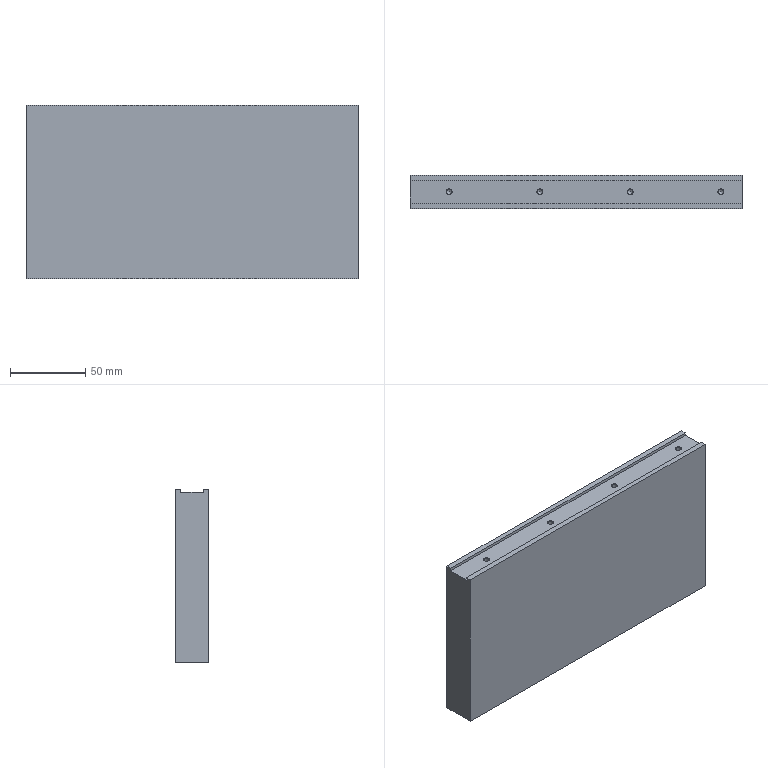Part | STEP file | Tube feed_id590_x_t | 1 solid | 22 faces | box 220 x 22 x 114.85 mm | volume 548747 mm3 | plane 10 | cone 8 | cylinder 4 | commonest cylinder face diameters 3.3 x4
STEP:
#1=CARTESIAN_POINT('',(0.,0.,0.));
#2=DIRECTION('',(0.,0.,1.));
#3=DIRECTION('',(1.,0.,0.));
#4=AXIS2_PLACEMENT_3D('',#1,#2,#3);
#5=CARTESIAN_POINT('',(21.,218.436,-89.15));
#6=VERTEX_POINT('',#5);
#7=CARTESIAN_POINT('',(21.,218.436,-91.15));
#8=VERTEX_POINT('',#7);
#9=CARTESIAN_POINT('',(21.,218.436,-89.969));
#10=DIRECTION('',(0.,0.,-1.));
#11=VECTOR('',#10,1.);
#12=LINE('',#9,#11);
#13=CARTESIAN_POINT('',(21.,221.936,-134.));
#14=DIRECTION('',(1.,0.,0.));
#15=DIRECTION('',(0.,0.,-1.));
#16=AXIS2_PLACEMENT_3D('',#13,#14,#15);
#17=PLANE('',#16);
#18=CARTESIAN_POINT('',(-44.031,-3.5));
#19=DIRECTION('',(1.,0.));
#20=VECTOR('',#19,1.);
#21=LINE('',#18,#20);
#22=(GEOMETRIC_REPRESENTATION_CONTEXT(2)PARAMETRIC_REPRESENTATION_CONTEXT()REPRESENTATION_CONTEXT('',''));
#23=DEFINITIONAL_REPRESENTATION('',(#21),#22);
#24=PCURVE('',#17,#23);
#25=CARTESIAN_POINT('',(1092.73,218.436,-89.969));
#26=DIRECTION('',(0.,1.,0.));
#27=DIRECTION('',(0.,0.,1.));
#28=AXIS2_PLACEMENT_3D('',#25,#26,#27);
#29=PLANE('',#28);
#30=CARTESIAN_POINT('',(0.,-1071.73));
#31=DIRECTION('',(-1.,0.));
#32=VECTOR('',#31,1.);
#33=LINE('',#30,#32);
#34=(GEOMETRIC_REPRESENTATION_CONTEXT(2)PARAMETRIC_REPRESENTATION_CONTEXT()REPRESENTATION_CONTEXT('',''));
#35=DEFINITIONAL_REPRESENTATION('',(#33),#34);
#36=PCURVE('',#29,#35);
#37=SURFACE_CURVE('',#12,(#24,#36),.PCURVE_S1.);
#38=EDGE_CURVE('',#6,#8,#37,.T.);
#39=ORIENTED_EDGE('',*,*,#38,.F.);
#40=CARTESIAN_POINT('',(21.,221.936,-89.15));
#41=VERTEX_POINT('',#40);
#42=CARTESIAN_POINT('',(21.,221.936,-89.15));
#43=DIRECTION('',(0.,-1.,0.));
#44=VECTOR('',#43,1.);
#45=LINE('',#42,#44);
#46=CARTESIAN_POINT('',(-44.85,0.));
#47=DIRECTION('',(0.,-1.));
#48=VECTOR('',#47,1.);
#49=LINE('',#46,#48);
#50=(GEOMETRIC_REPRESENTATION_CONTEXT(2)PARAMETRIC_REPRESENTATION_CONTEXT()REPRESENTATION_CONTEXT('',''));
#51=DEFINITIONAL_REPRESENTATION('',(#49),#50);
#52=PCURVE('',#17,#51);
#53=CARTESIAN_POINT('',(1092.73,218.436,-89.15));
#54=DIRECTION('',(0.,0.,-1.));
#55=DIRECTION('',(-1.,0.,0.));
#56=AXIS2_PLACEMENT_3D('',#53,#54,#55);
#57=PLANE('',#56);
#58=CARTESIAN_POINT('',(1071.73,3.5));
#59=DIRECTION('',(0.,-1.));
#60=VECTOR('',#59,1.);
#61=LINE('',#58,#60);
#62=(GEOMETRIC_REPRESENTATION_CONTEXT(2)PARAMETRIC_REPRESENTATION_CONTEXT()REPRESENTATION_CONTEXT('',''));
#63=DEFINITIONAL_REPRESENTATION('',(#61),#62);
#64=PCURVE('',#57,#63);
#65=SURFACE_CURVE('',#45,(#52,#64),.PCURVE_S1.);
#66=EDGE_CURVE('',#41,#6,#65,.T.);
#67=ORIENTED_EDGE('',*,*,#66,.F.);
#68=CARTESIAN_POINT('',(21.,221.936,-204.));
#69=VERTEX_POINT('',#68);
#70=CARTESIAN_POINT('',(21.,221.936,-134.));
#71=DIRECTION('',(0.,0.,-1.));
#72=VECTOR('',#71,1.);
#73=LINE('',#70,#72);
#74=CARTESIAN_POINT('',(0.,0.));
#75=DIRECTION('',(1.,0.));
#76=VECTOR('',#75,1.);
#77=LINE('',#74,#76);
#78=(GEOMETRIC_REPRESENTATION_CONTEXT(2)PARAMETRIC_REPRESENTATION_CONTEXT()REPRESENTATION_CONTEXT('',''));
#79=DEFINITIONAL_REPRESENTATION('',(#77),#78);
#80=PCURVE('',#17,#79);
#81=CARTESIAN_POINT('',(241.,221.936,-134.));
#82=DIRECTION('',(0.,-1.,0.));
#83=DIRECTION('',(0.,0.,-1.));
#84=AXIS2_PLACEMENT_3D('',#81,#82,#83);
#85=PLANE('',#84);
#86=CARTESIAN_POINT('',(0.,-220.));
#87=DIRECTION('',(1.,0.));
#88=VECTOR('',#87,1.);
#89=LINE('',#86,#88);
#90=(GEOMETRIC_REPRESENTATION_CONTEXT(2)PARAMETRIC_REPRESENTATION_CONTEXT()REPRESENTATION_CONTEXT('',''));
#91=DEFINITIONAL_REPRESENTATION('',(#89),#90);
#92=PCURVE('',#85,#91);
#93=SURFACE_CURVE('',#73,(#80,#92),.PCURVE_S1.);
#94=EDGE_CURVE('',#41,#69,#93,.T.);
#95=ORIENTED_EDGE('',*,*,#94,.T.);
#96=CARTESIAN_POINT('',(21.,199.936,-204.));
#97=VERTEX_POINT('',#96);
#98=CARTESIAN_POINT('',(21.,221.936,-204.));
#99=DIRECTION('',(0.,-1.,0.));
#100=VECTOR('',#99,1.);
#101=LINE('',#98,#100);
#102=CARTESIAN_POINT('',(70.,0.));
#103=DIRECTION('',(0.,-1.));
#104=VECTOR('',#103,1.);
#105=LINE('',#102,#104);
#106=(GEOMETRIC_REPRESENTATION_CONTEXT(2)PARAMETRIC_REPRESENTATION_CONTEXT()REPRESENTATION_CONTEXT('',''));
#107=DEFINITIONAL_REPRESENTATION('',(#105),#106);
#108=PCURVE('',#17,#107);
#109=CARTESIAN_POINT('',(0.,0.,-204.));
#110=DIRECTION('',(0.,0.,1.));
#111=DIRECTION('',(1.,0.,0.));
#112=AXIS2_PLACEMENT_3D('',#109,#110,#111);
#113=PLANE('',#112);
#114=CARTESIAN_POINT('',(21.,221.936));
#115=DIRECTION('',(0.,-1.));
#116=VECTOR('',#115,1.);
#117=LINE('',#114,#116);
#118=(GEOMETRIC_REPRESENTATION_CONTEXT(2)PARAMETRIC_REPRESENTATION_CONTEXT()REPRESENTATION_CONTEXT('',''));
#119=DEFINITIONAL_REPRESENTATION('',(#117),#118);
#120=PCURVE('',#113,#119);
#121=SURFACE_CURVE('',#101,(#108,#120),.PCURVE_S1.);
#122=EDGE_CURVE('',#69,#97,#121,.T.);
#123=ORIENTED_EDGE('',*,*,#122,.T.);
#124=CARTESIAN_POINT('',(21.,199.936,-89.15));
#125=VERTEX_POINT('',#124);
#126=CARTESIAN_POINT('',(21.,199.936,-134.));
#127=DIRECTION('',(0.,0.,-1.));
#128=VECTOR('',#127,1.);
#129=LINE('',#126,#128);
#130=CARTESIAN_POINT('',(0.,-22.));
#131=DIRECTION('',(1.,0.));
#132=VECTOR('',#131,1.);
#133=LINE('',#130,#132);
#134=(GEOMETRIC_REPRESENTATION_CONTEXT(2)PARAMETRIC_REPRESENTATION_CONTEXT()REPRESENTATION_CONTEXT('',''));
#135=DEFINITIONAL_REPRESENTATION('',(#133),#134);
#136=PCURVE('',#17,#135);
#137=CARTESIAN_POINT('',(21.,199.936,-134.));
#138=DIRECTION('',(0.,1.,0.));
#139=DIRECTION('',(0.,0.,1.));
#140=AXIS2_PLACEMENT_3D('',#137,#138,#139);
#141=PLANE('',#140);
#142=CARTESIAN_POINT('',(0.,0.));
#143=DIRECTION('',(-1.,0.));
#144=VECTOR('',#143,1.);
#145=LINE('',#142,#144);
#146=(GEOMETRIC_REPRESENTATION_CONTEXT(2)PARAMETRIC_REPRESENTATION_CONTEXT()REPRESENTATION_CONTEXT('',''));
#147=DEFINITIONAL_REPRESENTATION('',(#145),#146);
#148=PCURVE('',#141,#147);
#149=SURFACE_CURVE('',#129,(#136,#148),.PCURVE_S1.);
#150=EDGE_CURVE('',#125,#97,#149,.T.);
#151=ORIENTED_EDGE('',*,*,#150,.F.);
#152=CARTESIAN_POINT('',(21.,203.436,-89.15));
#153=VERTEX_POINT('',#152);
#154=CARTESIAN_POINT('',(21.,221.936,-89.15));
#155=DIRECTION('',(0.,-1.,0.));
#156=VECTOR('',#155,1.);
#157=LINE('',#154,#156);
#158=CARTESIAN_POINT('',(-44.85,0.));
#159=DIRECTION('',(0.,-1.));
#160=VECTOR('',#159,1.);
#161=LINE('',#158,#160);
#162=(GEOMETRIC_REPRESENTATION_CONTEXT(2)PARAMETRIC_REPRESENTATION_CONTEXT()REPRESENTATION_CONTEXT('',''));
#163=DEFINITIONAL_REPRESENTATION('',(#161),#162);
#164=PCURVE('',#17,#163);
#165=CARTESIAN_POINT('',(1092.73,218.436,-89.15));
#166=DIRECTION('',(0.,0.,-1.));
#167=DIRECTION('',(-1.,0.,0.));
#168=AXIS2_PLACEMENT_3D('',#165,#166,#167);
#169=PLANE('',#168);
#170=CARTESIAN_POINT('',(1071.73,3.5));
#171=DIRECTION('',(0.,-1.));
#172=VECTOR('',#171,1.);
#173=LINE('',#170,#172);
#174=(GEOMETRIC_REPRESENTATION_CONTEXT(2)PARAMETRIC_REPRESENTATION_CONTEXT()REPRESENTATION_CONTEXT('',''));
#175=DEFINITIONAL_REPRESENTATION('',(#173),#174);
#176=PCURVE('',#169,#175);
#177=SURFACE_CURVE('',#157,(#164,#176),.PCURVE_S1.);
#178=EDGE_CURVE('',#153,#125,#177,.T.);
#179=ORIENTED_EDGE('',*,*,#178,.F.);
#180=CARTESIAN_POINT('',(21.,203.436,-91.15));
#181=VERTEX_POINT('',#180);
#182=CARTESIAN_POINT('',(21.,203.436,-91.15));
#183=DIRECTION('',(0.,0.,1.));
#184=VECTOR('',#183,1.);
#185=LINE('',#182,#184);
#186=CARTESIAN_POINT('',(-42.85,-18.5));
#187=DIRECTION('',(-1.,0.));
#188=VECTOR('',#187,1.);
#189=LINE('',#186,#188);
#190=(GEOMETRIC_REPRESENTATION_CONTEXT(2)PARAMETRIC_REPRESENTATION_CONTEXT()REPRESENTATION_CONTEXT('',''));
#191=DEFINITIONAL_REPRESENTATION('',(#189),#190);
#192=PCURVE('',#17,#191);
#193=CARTESIAN_POINT('',(1092.73,203.436,-91.15));
#194=DIRECTION('',(0.,-1.,0.));
#195=DIRECTION('',(0.,0.,-1.));
#196=AXIS2_PLACEMENT_3D('',#193,#194,#195);
#197=PLANE('',#196);
#198=CARTESIAN_POINT('',(0.,-1071.73));
#199=DIRECTION('',(-1.,0.));
#200=VECTOR('',#199,1.);
#201=LINE('',#198,#200);
#202=(GEOMETRIC_REPRESENTATION_CONTEXT(2)PARAMETRIC_REPRESENTATION_CONTEXT()REPRESENTATION_CONTEXT('',''));
#203=DEFINITIONAL_REPRESENTATION('',(#201),#202);
#204=PCURVE('',#197,#203);
#205=SURFACE_CURVE('',#185,(#192,#204),.PCURVE_S1.);
#206=EDGE_CURVE('',#181,#153,#205,.T.);
#207=ORIENTED_EDGE('',*,*,#206,.F.);
#208=CARTESIAN_POINT('',(21.,218.436,-91.15));
#209=DIRECTION('',(0.,-1.,0.));
#210=VECTOR('',#209,1.);
#211=LINE('',#208,#210);
#212=CARTESIAN_POINT('',(-42.85,-3.5));
#213=DIRECTION('',(0.,-1.));
#214=VECTOR('',#213,1.);
#215=LINE('',#212,#214);
#216=(GEOMETRIC_REPRESENTATION_CONTEXT(2)PARAMETRIC_REPRESENTATION_CONTEXT()REPRESENTATION_CONTEXT('',''));
#217=DEFINITIONAL_REPRESENTATION('',(#215),#216);
#218=PCURVE('',#17,#217);
#219=CARTESIAN_POINT('',(1092.73,218.436,-91.15));
#220=DIRECTION('',(0.,0.,-1.));
#221=DIRECTION('',(-1.,0.,0.));
#222=AXIS2_PLACEMENT_3D('',#219,#220,#221);
#223=PLANE('',#222);
#224=CARTESIAN_POINT('',(1071.73,0.));
#225=DIRECTION('',(0.,-1.));
#226=VECTOR('',#225,1.);
#227=LINE('',#224,#226);
#228=(GEOMETRIC_REPRESENTATION_CONTEXT(2)PARAMETRIC_REPRESENTATION_CONTEXT()REPRESENTATION_CONTEXT('',''));
#229=DEFINITIONAL_REPRESENTATION('',(#227),#228);
#230=PCURVE('',#223,#229);
#231=SURFACE_CURVE('',#211,(#218,#230),.PCURVE_S1.);
#232=EDGE_CURVE('',#8,#181,#231,.T.);
#233=ORIENTED_EDGE('',*,*,#232,.F.);
#234=EDGE_LOOP('',(#39,#67,#95,#123,#151,#179,#207,#233));
#235=FACE_BOUND('',#234,.T.);
#236=ADVANCED_FACE('',(#235),#17,.F.);
#237=CARTESIAN_POINT('',(241.,203.436,-89.15));
#238=VERTEX_POINT('',#237);
#239=CARTESIAN_POINT('',(241.,203.436,-91.15));
#240=VERTEX_POINT('',#239);
#241=CARTESIAN_POINT('',(241.,203.436,-91.15));
#242=DIRECTION('',(0.,0.,-1.));
#243=VECTOR('',#242,1.);
#244=LINE('',#241,#243);
#245=CARTESIAN_POINT('',(241.,199.936,-134.));
#246=DIRECTION('',(-1.,0.,0.));
#247=DIRECTION('',(0.,0.,1.));
#248=AXIS2_PLACEMENT_3D('',#245,#246,#247);
#249=PLANE('',#248);
#250=CARTESIAN_POINT('',(42.85,3.5));
#251=DIRECTION('',(-1.,0.));
#252=VECTOR('',#251,1.);
#253=LINE('',#250,#252);
#254=(GEOMETRIC_REPRESENTATION_CONTEXT(2)PARAMETRIC_REPRESENTATION_CONTEXT()REPRESENTATION_CONTEXT('',''));
#255=DEFINITIONAL_REPRESENTATION('',(#253),#254);
#256=PCURVE('',#249,#255);
#257=CARTESIAN_POINT('',(0.,-851.73));
#258=DIRECTION('',(1.,0.));
#259=VECTOR('',#258,1.);
#260=LINE('',#257,#259);
#261=(GEOMETRIC_REPRESENTATION_CONTEXT(2)PARAMETRIC_REPRESENTATION_CONTEXT()REPRESENTATION_CONTEXT('',''));
#262=DEFINITIONAL_REPRESENTATION('',(#260),#261);
#263=PCURVE('',#197,#262);
#264=SURFACE_CURVE('',#244,(#256,#263),.PCURVE_S1.);
#265=EDGE_CURVE('',#238,#240,#264,.T.);
#266=ORIENTED_EDGE('',*,*,#265,.F.);
#267=CARTESIAN_POINT('',(241.,199.936,-89.15));
#268=VERTEX_POINT('',#267);
#269=CARTESIAN_POINT('',(241.,199.936,-89.15));
#270=DIRECTION('',(0.,1.,0.));
#271=VECTOR('',#270,1.);
#272=LINE('',#269,#271);
#273=CARTESIAN_POINT('',(44.85,0.));
#274=DIRECTION('',(0.,1.));
#275=VECTOR('',#274,1.);
#276=LINE('',#273,#275);
#277=(GEOMETRIC_REPRESENTATION_CONTEXT(2)PARAMETRIC_REPRESENTATION_CONTEXT()REPRESENTATION_CONTEXT('',''));
#278=DEFINITIONAL_REPRESENTATION('',(#276),#277);
#279=PCURVE('',#249,#278);
#280=CARTESIAN_POINT('',(851.73,-18.5));
#281=DIRECTION('',(0.,1.));
#282=VECTOR('',#281,1.);
#283=LINE('',#280,#282);
#284=(GEOMETRIC_REPRESENTATION_CONTEXT(2)PARAMETRIC_REPRESENTATION_CONTEXT()REPRESENTATION_CONTEXT('',''));
#285=DEFINITIONAL_REPRESENTATION('',(#283),#284);
#286=PCURVE('',#169,#285);
#287=SURFACE_CURVE('',#272,(#279,#286),.PCURVE_S1.);
#288=EDGE_CURVE('',#268,#238,#287,.T.);
#289=ORIENTED_EDGE('',*,*,#288,.F.);
#290=CARTESIAN_POINT('',(241.,199.936,-204.));
#291=VERTEX_POINT('',#290);
#292=CARTESIAN_POINT('',(241.,199.936,-134.));
#293=DIRECTION('',(0.,0.,-1.));
#294=VECTOR('',#293,1.);
#295=LINE('',#292,#294);
#296=CARTESIAN_POINT('',(0.,0.));
#297=DIRECTION('',(-1.,0.));
#298=VECTOR('',#297,1.);
#299=LINE('',#296,#298);
#300=(GEOMETRIC_REPRESENTATION_CONTEXT(2)PARAMETRIC_REPRESENTATION_CONTEXT()REPRESENTATION_CONTEXT('',''));
#301=DEFINITIONAL_REPRESENTATION('',(#299),#300);
#302=PCURVE('',#249,#301);
#303=CARTESIAN_POINT('',(0.,220.));
#304=DIRECTION('',(-1.,0.));
#305=VECTOR('',#304,1.);
#306=LINE('',#303,#305);
#307=(GEOMETRIC_REPRESENTATION_CONTEXT(2)PARAMETRIC_REPRESENTATION_CONTEXT()REPRESENTATION_CONTEXT('',''));
#308=DEFINITIONAL_REPRESENTATION('',(#306),#307);
#309=PCURVE('',#141,#308);
#310=SURFACE_CURVE('',#295,(#302,#309),.PCURVE_S1.);
#311=EDGE_CURVE('',#268,#291,#310,.T.);
#312=ORIENTED_EDGE('',*,*,#311,.T.);
#313=CARTESIAN_POINT('',(241.,221.936,-204.));
#314=VERTEX_POINT('',#313);
#315=CARTESIAN_POINT('',(241.,199.936,-204.));
#316=DIRECTION('',(0.,1.,0.));
#317=VECTOR('',#316,1.);
#318=LINE('',#315,#317);
#319=CARTESIAN_POINT('',(-70.,0.));
#320=DIRECTION('',(0.,1.));
#321=VECTOR('',#320,1.);
#322=LINE('',#319,#321);
#323=(GEOMETRIC_REPRESENTATION_CONTEXT(2)PARAMETRIC_REPRESENTATION_CONTEXT()REPRESENTATION_CONTEXT('',''));
#324=DEFINITIONAL_REPRESENTATION('',(#322),#323);
#325=PCURVE('',#249,#324);
#326=CARTESIAN_POINT('',(241.,199.936));
#327=DIRECTION('',(0.,1.));
#328=VECTOR('',#327,1.);
#329=LINE('',#326,#328);
#330=(GEOMETRIC_REPRESENTATION_CONTEXT(2)PARAMETRIC_REPRESENTATION_CONTEXT()REPRESENTATION_CONTEXT('',''));
#331=DEFINITIONAL_REPRESENTATION('',(#329),#330);
#332=PCURVE('',#113,#331);
#333=SURFACE_CURVE('',#318,(#325,#332),.PCURVE_S1.);
#334=EDGE_CURVE('',#291,#314,#333,.T.);
#335=ORIENTED_EDGE('',*,*,#334,.T.);
#336=CARTESIAN_POINT('',(241.,221.936,-89.15));
#337=VERTEX_POINT('',#336);
#338=CARTESIAN_POINT('',(241.,221.936,-134.));
#339=DIRECTION('',(0.,0.,-1.));
#340=VECTOR('',#339,1.);
#341=LINE('',#338,#340);
#342=CARTESIAN_POINT('',(0.,22.));
#343=DIRECTION('',(-1.,0.));
#344=VECTOR('',#343,1.);
#345=LINE('',#342,#344);
#346=(GEOMETRIC_REPRESENTATION_CONTEXT(2)PARAMETRIC_REPRESENTATION_CONTEXT()REPRESENTATION_CONTEXT('',''));
#347=DEFINITIONAL_REPRESENTATION('',(#345),#346);
#348=PCURVE('',#249,#347);
#349=CARTESIAN_POINT('',(0.,0.));
#350=DIRECTION('',(1.,0.));
#351=VECTOR('',#350,1.);
#352=LINE('',#349,#351);
#353=(GEOMETRIC_REPRESENTATION_CONTEXT(2)PARAMETRIC_REPRESENTATION_CONTEXT()REPRESENTATION_CONTEXT('',''));
#354=DEFINITIONAL_REPRESENTATION('',(#352),#353);
#355=PCURVE('',#85,#354);
#356=SURFACE_CURVE('',#341,(#348,#355),.PCURVE_S1.);
#357=EDGE_CURVE('',#337,#314,#356,.T.);
#358=ORIENTED_EDGE('',*,*,#357,.F.);
#359=CARTESIAN_POINT('',(241.,218.436,-89.15));
#360=VERTEX_POINT('',#359);
#361=CARTESIAN_POINT('',(241.,199.936,-89.15));
#362=DIRECTION('',(0.,1.,0.));
#363=VECTOR('',#362,1.);
#364=LINE('',#361,#363);
#365=CARTESIAN_POINT('',(44.85,0.));
#366=DIRECTION('',(0.,1.));
#367=VECTOR('',#366,1.);
#368=LINE('',#365,#367);
#369=(GEOMETRIC_REPRESENTATION_CONTEXT(2)PARAMETRIC_REPRESENTATION_CONTEXT()REPRESENTATION_CONTEXT('',''));
#370=DEFINITIONAL_REPRESENTATION('',(#368),#369);
#371=PCURVE('',#249,#370);
#372=CARTESIAN_POINT('',(851.73,-18.5));
#373=DIRECTION('',(0.,1.));
#374=VECTOR('',#373,1.);
#375=LINE('',#372,#374);
#376=(GEOMETRIC_REPRESENTATION_CONTEXT(2)PARAMETRIC_REPRESENTATION_CONTEXT()REPRESENTATION_CONTEXT('',''));
#377=DEFINITIONAL_REPRESENTATION('',(#375),#376);
#378=PCURVE('',#57,#377);
#379=SURFACE_CURVE('',#364,(#371,#378),.PCURVE_S1.);
#380=EDGE_CURVE('',#360,#337,#379,.T.);
#381=ORIENTED_EDGE('',*,*,#380,.F.);
#382=CARTESIAN_POINT('',(241.,218.436,-91.15));
#383=VERTEX_POINT('',#382);
#384=CARTESIAN_POINT('',(241.,218.436,-89.969));
#385=DIRECTION('',(0.,0.,1.));
#386=VECTOR('',#385,1.);
#387=LINE('',#384,#386);
#388=CARTESIAN_POINT('',(44.031,18.5));
#389=DIRECTION('',(1.,0.));
#390=VECTOR('',#389,1.);
#391=LINE('',#388,#390);
#392=(GEOMETRIC_REPRESENTATION_CONTEXT(2)PARAMETRIC_REPRESENTATION_CONTEXT()REPRESENTATION_CONTEXT('',''));
#393=DEFINITIONAL_REPRESENTATION('',(#391),#392);
#394=PCURVE('',#249,#393);
#395=CARTESIAN_POINT('',(0.,-851.73));
#396=DIRECTION('',(1.,0.));
#397=VECTOR('',#396,1.);
#398=LINE('',#395,#397);
#399=(GEOMETRIC_REPRESENTATION_CONTEXT(2)PARAMETRIC_REPRESENTATION_CONTEXT()REPRESENTATION_CONTEXT('',''));
#400=DEFINITIONAL_REPRESENTATION('',(#398),#399);
#401=PCURVE('',#29,#400);
#402=SURFACE_CURVE('',#387,(#394,#401),.PCURVE_S1.);
#403=EDGE_CURVE('',#383,#360,#402,.T.);
#404=ORIENTED_EDGE('',*,*,#403,.F.);
#405=CARTESIAN_POINT('',(241.,218.436,-91.15));
#406=DIRECTION('',(0.,1.,0.));
#407=VECTOR('',#406,1.);
#408=LINE('',#405,#407);
#409=CARTESIAN_POINT('',(42.85,18.5));
#410=DIRECTION('',(0.,1.));
#411=VECTOR('',#410,1.);
#412=LINE('',#409,#411);
#413=(GEOMETRIC_REPRESENTATION_CONTEXT(2)PARAMETRIC_REPRESENTATION_CONTEXT()REPRESENTATION_CONTEXT('',''));
#414=DEFINITIONAL_REPRESENTATION('',(#412),#413);
#415=PCURVE('',#249,#414);
#416=CARTESIAN_POINT('',(851.73,0.));
#417=DIRECTION('',(0.,1.));
#418=VECTOR('',#417,1.);
#419=LINE('',#416,#418);
#420=(GEOMETRIC_REPRESENTATION_CONTEXT(2)PARAMETRIC_REPRESENTATION_CONTEXT()REPRESENTATION_CONTEXT('',''));
#421=DEFINITIONAL_REPRESENTATION('',(#419),#420);
#422=PCURVE('',#223,#421);
#423=SURFACE_CURVE('',#408,(#415,#422),.PCURVE_S1.);
#424=EDGE_CURVE('',#240,#383,#423,.T.);
#425=ORIENTED_EDGE('',*,*,#424,.F.);
#426=EDGE_LOOP('',(#266,#289,#312,#335,#358,#381,#404,#425));
#427=FACE_BOUND('',#426,.T.);
#428=ADVANCED_FACE('',(#427),#249,.F.);
#429=CARTESIAN_POINT('',(1092.73,203.436,-89.15));
#430=DIRECTION('',(1.,0.,0.));
#431=VECTOR('',#430,1.);
#432=LINE('',#429,#431);
#433=CARTESIAN_POINT('',(0.,-15.));
#434=DIRECTION('',(-1.,0.));
#435=VECTOR('',#434,1.);
#436=LINE('',#433,#435);
#437=(GEOMETRIC_REPRESENTATION_CONTEXT(2)PARAMETRIC_REPRESENTATION_CONTEXT()REPRESENTATION_CONTEXT('',''));
#438=DEFINITIONAL_REPRESENTATION('',(#436),#437);
#439=PCURVE('',#169,#438);
#440=CARTESIAN_POINT('',(-2.,0.));
#441=DIRECTION('',(0.,1.));
#442=VECTOR('',#441,1.);
#443=LINE('',#440,#442);
#444=(GEOMETRIC_REPRESENTATION_CONTEXT(2)PARAMETRIC_REPRESENTATION_CONTEXT()REPRESENTATION_CONTEXT('',''));
#445=DEFINITIONAL_REPRESENTATION('',(#443),#444);
#446=PCURVE('',#197,#445);
#447=SURFACE_CURVE('',#432,(#439,#446),.PCURVE_S1.);
#448=EDGE_CURVE('',#153,#238,#447,.T.);
#449=ORIENTED_EDGE('',*,*,#448,.F.);
#450=ORIENTED_EDGE('',*,*,#178,.T.);
#451=CARTESIAN_POINT('',(21.,199.936,-89.15));
#452=DIRECTION('',(1.,0.,0.));
#453=VECTOR('',#452,1.);
#454=LINE('',#451,#453);
#455=CARTESIAN_POINT('',(1071.73,-18.5));
#456=DIRECTION('',(-1.,0.));
#457=VECTOR('',#456,1.);
#458=LINE('',#455,#457);
#459=(GEOMETRIC_REPRESENTATION_CONTEXT(2)PARAMETRIC_REPRESENTATION_CONTEXT()REPRESENTATION_CONTEXT('',''));
#460=DEFINITIONAL_REPRESENTATION('',(#458),#459);
#461=PCURVE('',#169,#460);
#462=CARTESIAN_POINT('',(44.85,0.));
#463=DIRECTION('',(0.,1.));
#464=VECTOR('',#463,1.);
#465=LINE('',#462,#464);
#466=(GEOMETRIC_REPRESENTATION_CONTEXT(2)PARAMETRIC_REPRESENTATION_CONTEXT()REPRESENTATION_CONTEXT('',''));
#467=DEFINITIONAL_REPRESENTATION('',(#465),#466);
#468=PCURVE('',#141,#467);
#469=SURFACE_CURVE('',#454,(#461,#468),.PCURVE_S1.);
#470=EDGE_CURVE('',#125,#268,#469,.T.);
#471=ORIENTED_EDGE('',*,*,#470,.T.);
#472=ORIENTED_EDGE('',*,*,#288,.T.);
#473=EDGE_LOOP('',(#449,#450,#471,#472));
#474=FACE_BOUND('',#473,.T.);
#475=ADVANCED_FACE('',(#474),#169,.F.);
#476=CARTESIAN_POINT('',(21.,199.936,-204.));
#477=DIRECTION('',(1.,0.,0.));
#478=VECTOR('',#477,1.);
#479=LINE('',#476,#478);
#480=CARTESIAN_POINT('',(-70.,0.));
#481=DIRECTION('',(0.,1.));
#482=VECTOR('',#481,1.);
#483=LINE('',#480,#482);
#484=(GEOMETRIC_REPRESENTATION_CONTEXT(2)PARAMETRIC_REPRESENTATION_CONTEXT()REPRESENTATION_CONTEXT('',''));
#485=DEFINITIONAL_REPRESENTATION('',(#483),#484);
#486=PCURVE('',#141,#485);
#487=CARTESIAN_POINT('',(21.,199.936));
#488=DIRECTION('',(1.,0.));
#489=VECTOR('',#488,1.);
#490=LINE('',#487,#489);
#491=(GEOMETRIC_REPRESENTATION_CONTEXT(2)PARAMETRIC_REPRESENTATION_CONTEXT()REPRESENTATION_CONTEXT('',''));
#492=DEFINITIONAL_REPRESENTATION('',(#490),#491);
#493=PCURVE('',#113,#492);
#494=SURFACE_CURVE('',#479,(#486,#493),.PCURVE_S1.);
#495=EDGE_CURVE('',#97,#291,#494,.T.);
#496=ORIENTED_EDGE('',*,*,#495,.T.);
#497=ORIENTED_EDGE('',*,*,#311,.F.);
#498=ORIENTED_EDGE('',*,*,#470,.F.);
#499=ORIENTED_EDGE('',*,*,#150,.T.);
#500=EDGE_LOOP('',(#496,#497,#498,#499));
#501=FACE_BOUND('',#500,.T.);
#502=ADVANCED_FACE('',(#501),#141,.F.);
#503=CARTESIAN_POINT('',(241.,221.936,-204.));
#504=DIRECTION('',(-1.,0.,0.));
#505=VECTOR('',#504,1.);
#506=LINE('',#503,#505);
#507=CARTESIAN_POINT('',(70.,0.));
#508=DIRECTION('',(0.,-1.));
#509=VECTOR('',#508,1.);
#510=LINE('',#507,#509);
#511=(GEOMETRIC_REPRESENTATION_CONTEXT(2)PARAMETRIC_REPRESENTATION_CONTEXT()REPRESENTATION_CONTEXT('',''));
#512=DEFINITIONAL_REPRESENTATION('',(#510),#511);
#513=PCURVE('',#85,#512);
#514=CARTESIAN_POINT('',(241.,221.936));
#515=DIRECTION('',(-1.,0.));
#516=VECTOR('',#515,1.);
#517=LINE('',#514,#516);
#518=(GEOMETRIC_REPRESENTATION_CONTEXT(2)PARAMETRIC_REPRESENTATION_CONTEXT()REPRESENTATION_CONTEXT('',''));
#519=DEFINITIONAL_REPRESENTATION('',(#517),#518);
#520=PCURVE('',#113,#519);
#521=SURFACE_CURVE('',#506,(#513,#520),.PCURVE_S1.);
#522=EDGE_CURVE('',#314,#69,#521,.T.);
#523=ORIENTED_EDGE('',*,*,#522,.T.);
#524=ORIENTED_EDGE('',*,*,#94,.F.);
#525=CARTESIAN_POINT('',(241.,221.936,-89.15));
#526=DIRECTION('',(-1.,0.,0.));
#527=VECTOR('',#526,1.);
#528=LINE('',#525,#527);
#529=CARTESIAN_POINT('',(-44.85,0.));
#530=DIRECTION('',(0.,-1.));
#531=VECTOR('',#530,1.);
#532=LINE('',#529,#531);
#533=(GEOMETRIC_REPRESENTATION_CONTEXT(2)PARAMETRIC_REPRESENTATION_CONTEXT()REPRESENTATION_CONTEXT('',''));
#534=DEFINITIONAL_REPRESENTATION('',(#532),#533);
#535=PCURVE('',#85,#534);
#536=CARTESIAN_POINT('',(851.73,3.5));
#537=DIRECTION('',(1.,0.));
#538=VECTOR('',#537,1.);
#539=LINE('',#536,#538);
#540=(GEOMETRIC_REPRESENTATION_CONTEXT(2)PARAMETRIC_REPRESENTATION_CONTEXT()REPRESENTATION_CONTEXT('',''));
#541=DEFINITIONAL_REPRESENTATION('',(#539),#540);
#542=PCURVE('',#57,#541);
#543=SURFACE_CURVE('',#528,(#535,#542),.PCURVE_S1.);
#544=EDGE_CURVE('',#337,#41,#543,.T.);
#545=ORIENTED_EDGE('',*,*,#544,.F.);
#546=ORIENTED_EDGE('',*,*,#357,.T.);
#547=EDGE_LOOP('',(#523,#524,#545,#546));
#548=FACE_BOUND('',#547,.T.);
#549=ADVANCED_FACE('',(#548),#85,.F.);
#550=CARTESIAN_POINT('',(1092.73,218.436,-89.15));
#551=DIRECTION('',(-1.,0.,0.));
#552=VECTOR('',#551,1.);
#553=LINE('',#550,#552);
#554=CARTESIAN_POINT('',(0.,0.));
#555=DIRECTION('',(1.,0.));
#556=VECTOR('',#555,1.);
#557=LINE('',#554,#556);
#558=(GEOMETRIC_REPRESENTATION_CONTEXT(2)PARAMETRIC_REPRESENTATION_CONTEXT()REPRESENTATION_CONTEXT('',''));
#559=DEFINITIONAL_REPRESENTATION('',(#557),#558);
#560=PCURVE('',#57,#559);
#561=CARTESIAN_POINT('',(0.8185,0.));
#562=DIRECTION('',(0.,-1.));
#563=VECTOR('',#562,1.);
#564=LINE('',#561,#563);
#565=(GEOMETRIC_REPRESENTATION_CONTEXT(2)PARAMETRIC_REPRESENTATION_CONTEXT()REPRESENTATION_CONTEXT('',''));
#566=DEFINITIONAL_REPRESENTATION('',(#564),#565);
#567=PCURVE('',#29,#566);
#568=SURFACE_CURVE('',#553,(#560,#567),.PCURVE_S1.);
#569=EDGE_CURVE('',#360,#6,#568,.T.);
#570=ORIENTED_EDGE('',*,*,#569,.F.);
#571=ORIENTED_EDGE('',*,*,#380,.T.);
#572=ORIENTED_EDGE('',*,*,#544,.T.);
#573=ORIENTED_EDGE('',*,*,#66,.T.);
#574=EDGE_LOOP('',(#570,#571,#572,#573));
#575=FACE_BOUND('',#574,.T.);
#576=ADVANCED_FACE('',(#575),#57,.F.);
#577=ORIENTED_EDGE('',*,*,#122,.F.);
#578=ORIENTED_EDGE('',*,*,#522,.F.);
#579=ORIENTED_EDGE('',*,*,#334,.F.);
#580=ORIENTED_EDGE('',*,*,#495,.F.);
#581=EDGE_LOOP('',(#577,#578,#579,#580));
#582=FACE_BOUND('',#581,.T.);
#583=ADVANCED_FACE('',(#582),#113,.F.);
#584=ORIENTED_EDGE('',*,*,#448,.T.);
#585=ORIENTED_EDGE('',*,*,#265,.T.);
#586=CARTESIAN_POINT('',(1092.73,203.436,-91.15));
#587=DIRECTION('',(1.,0.,0.));
#588=VECTOR('',#587,1.);
#589=LINE('',#586,#588);
#590=CARTESIAN_POINT('',(0.,0.));
#591=DIRECTION('',(0.,1.));
#592=VECTOR('',#591,1.);
#593=LINE('',#590,#592);
#594=(GEOMETRIC_REPRESENTATION_CONTEXT(2)PARAMETRIC_REPRESENTATION_CONTEXT()REPRESENTATION_CONTEXT('',''));
#595=DEFINITIONAL_REPRESENTATION('',(#593),#594);
#596=PCURVE('',#197,#595);
#597=CARTESIAN_POINT('',(0.,-15.));
#598=DIRECTION('',(-1.,0.));
#599=VECTOR('',#598,1.);
#600=LINE('',#597,#599);
#601=(GEOMETRIC_REPRESENTATION_CONTEXT(2)PARAMETRIC_REPRESENTATION_CONTEXT()REPRESENTATION_CONTEXT('',''));
#602=DEFINITIONAL_REPRESENTATION('',(#600),#601);
#603=PCURVE('',#223,#602);
#604=SURFACE_CURVE('',#589,(#596,#603),.PCURVE_S1.);
#605=EDGE_CURVE('',#181,#240,#604,.T.);
#606=ORIENTED_EDGE('',*,*,#605,.F.);
#607=ORIENTED_EDGE('',*,*,#206,.T.);
#608=EDGE_LOOP('',(#584,#585,#606,#607));
#609=FACE_BOUND('',#608,.T.);
#610=ADVANCED_FACE('',(#609),#197,.F.);
#611=ORIENTED_EDGE('',*,*,#569,.T.);
#612=ORIENTED_EDGE('',*,*,#38,.T.);
#613=CARTESIAN_POINT('',(1092.73,218.436,-91.15));
#614=DIRECTION('',(1.,0.,0.));
#615=VECTOR('',#614,1.);
#616=LINE('',#613,#615);
#617=CARTESIAN_POINT('',(-1.181,0.));
#618=DIRECTION('',(0.,1.));
#619=VECTOR('',#618,1.);
#620=LINE('',#617,#619);
#621=(GEOMETRIC_REPRESENTATION_CONTEXT(2)PARAMETRIC_REPRESENTATION_CONTEXT()REPRESENTATION_CONTEXT('',''));
#622=DEFINITIONAL_REPRESENTATION('',(#620),#621);
#623=PCURVE('',#29,#622);
#624=CARTESIAN_POINT('',(0.,0.));
#625=DIRECTION('',(-1.,0.));
#626=VECTOR('',#625,1.);
#627=LINE('',#624,#626);
#628=(GEOMETRIC_REPRESENTATION_CONTEXT(2)PARAMETRIC_REPRESENTATION_CONTEXT()REPRESENTATION_CONTEXT('',''));
#629=DEFINITIONAL_REPRESENTATION('',(#627),#628);
#630=PCURVE('',#223,#629);
#631=SURFACE_CURVE('',#616,(#623,#630),.PCURVE_S1.);
#632=EDGE_CURVE('',#8,#383,#631,.T.);
#633=ORIENTED_EDGE('',*,*,#632,.T.);
#634=ORIENTED_EDGE('',*,*,#403,.T.);
#635=EDGE_LOOP('',(#611,#612,#633,#634));
#636=FACE_BOUND('',#635,.T.);
#637=ADVANCED_FACE('',(#636),#29,.F.);
#638=CARTESIAN_POINT('',(224.982,210.936,-91.15));
#639=VERTEX_POINT('',#638);
#640=CARTESIAN_POINT('',(226.982,210.936,-91.15));
#641=DIRECTION('',(0.,0.,-1.));
#642=DIRECTION('',(-1.,0.,0.));
#643=AXIS2_PLACEMENT_3D('',#640,#641,#642);
#644=CIRCLE('',#643,2.);
#645=CARTESIAN_POINT('',(865.748,-7.5));
#646=DIRECTION('',(1.,0.));
#647=AXIS2_PLACEMENT_2D('',#645,#646);
#648=CIRCLE('',#647,2.);
#649=(GEOMETRIC_REPRESENTATION_CONTEXT(2)PARAMETRIC_REPRESENTATION_CONTEXT()REPRESENTATION_CONTEXT('',''));
#650=DEFINITIONAL_REPRESENTATION('',(#648),#649);
#651=PCURVE('',#223,#650);
#652=CARTESIAN_POINT('',(226.982,210.936,-91.15));
#653=DIRECTION('',(0.,0.,1.));
#654=DIRECTION('',(1.,0.,0.));
#655=AXIS2_PLACEMENT_3D('',#652,#653,#654);
#656=CONICAL_SURFACE('',#655,2.,0.7854);
#657=CARTESIAN_POINT('',(9.425,0.));
#658=DIRECTION('',(-1.,0.));
#659=VECTOR('',#658,1.);
#660=LINE('',#657,#659);
#661=(GEOMETRIC_REPRESENTATION_CONTEXT(2)PARAMETRIC_REPRESENTATION_CONTEXT()REPRESENTATION_CONTEXT('',''));
#662=DEFINITIONAL_REPRESENTATION('',(#660),#661);
#663=PCURVE('',#656,#662);
#664=SURFACE_CURVE('',#644,(#651,#663),.PCURVE_S1.);
#665=EDGE_CURVE('',#639,#639,#664,.T.);
#666=ORIENTED_EDGE('',*,*,#665,.T.);
#667=EDGE_LOOP('',(#666));
#668=FACE_BOUND('',#667,.T.);
#669=CARTESIAN_POINT('',(164.982,210.936,-91.15));
#670=VERTEX_POINT('',#669);
#671=CARTESIAN_POINT('',(166.982,210.936,-91.15));
#672=DIRECTION('',(0.,0.,-1.));
#673=DIRECTION('',(-1.,0.,0.));
#674=AXIS2_PLACEMENT_3D('',#671,#672,#673);
#675=CIRCLE('',#674,2.);
#676=CARTESIAN_POINT('',(925.748,-7.5));
#677=DIRECTION('',(1.,0.));
#678=AXIS2_PLACEMENT_2D('',#676,#677);
#679=CIRCLE('',#678,2.);
#680=(GEOMETRIC_REPRESENTATION_CONTEXT(2)PARAMETRIC_REPRESENTATION_CONTEXT()REPRESENTATION_CONTEXT('',''));
#681=DEFINITIONAL_REPRESENTATION('',(#679),#680);
#682=PCURVE('',#223,#681);
#683=CARTESIAN_POINT('',(166.982,210.936,-91.15));
#684=DIRECTION('',(0.,0.,1.));
#685=DIRECTION('',(1.,0.,0.));
#686=AXIS2_PLACEMENT_3D('',#683,#684,#685);
#687=CONICAL_SURFACE('',#686,2.,0.7854);
#688=CARTESIAN_POINT('',(9.425,0.));
#689=DIRECTION('',(-1.,0.));
#690=VECTOR('',#689,1.);
#691=LINE('',#688,#690);
#692=(GEOMETRIC_REPRESENTATION_CONTEXT(2)PARAMETRIC_REPRESENTATION_CONTEXT()REPRESENTATION_CONTEXT('',''));
#693=DEFINITIONAL_REPRESENTATION('',(#691),#692);
#694=PCURVE('',#687,#693);
#695=SURFACE_CURVE('',#675,(#682,#694),.PCURVE_S1.);
#696=EDGE_CURVE('',#670,#670,#695,.T.);
#697=ORIENTED_EDGE('',*,*,#696,.T.);
#698=EDGE_LOOP('',(#697));
#699=FACE_BOUND('',#698,.T.);
#700=CARTESIAN_POINT('',(104.982,210.936,-91.15));
#701=VERTEX_POINT('',#700);
#702=CARTESIAN_POINT('',(106.982,210.936,-91.15));
#703=DIRECTION('',(0.,0.,-1.));
#704=DIRECTION('',(-1.,0.,0.));
#705=AXIS2_PLACEMENT_3D('',#702,#703,#704);
#706=CIRCLE('',#705,2.);
#707=CARTESIAN_POINT('',(985.748,-7.5));
#708=DIRECTION('',(1.,0.));
#709=AXIS2_PLACEMENT_2D('',#707,#708);
#710=CIRCLE('',#709,2.);
#711=(GEOMETRIC_REPRESENTATION_CONTEXT(2)PARAMETRIC_REPRESENTATION_CONTEXT()REPRESENTATION_CONTEXT('',''));
#712=DEFINITIONAL_REPRESENTATION('',(#710),#711);
#713=PCURVE('',#223,#712);
#714=CARTESIAN_POINT('',(106.982,210.936,-91.15));
#715=DIRECTION('',(0.,0.,1.));
#716=DIRECTION('',(1.,0.,0.));
#717=AXIS2_PLACEMENT_3D('',#714,#715,#716);
#718=CONICAL_SURFACE('',#717,2.,0.7854);
#719=CARTESIAN_POINT('',(9.425,0.));
#720=DIRECTION('',(-1.,0.));
#721=VECTOR('',#720,1.);
#722=LINE('',#719,#721);
#723=(GEOMETRIC_REPRESENTATION_CONTEXT(2)PARAMETRIC_REPRESENTATION_CONTEXT()REPRESENTATION_CONTEXT('',''));
#724=DEFINITIONAL_REPRESENTATION('',(#722),#723);
#725=PCURVE('',#718,#724);
#726=SURFACE_CURVE('',#706,(#713,#725),.PCURVE_S1.);
#727=EDGE_CURVE('',#701,#701,#726,.T.);
#728=ORIENTED_EDGE('',*,*,#727,.T.);
#729=EDGE_LOOP('',(#728));
#730=FACE_BOUND('',#729,.T.);
#731=CARTESIAN_POINT('',(44.982,210.936,-91.15));
#732=VERTEX_POINT('',#731);
#733=CARTESIAN_POINT('',(46.982,210.936,-91.15));
#734=DIRECTION('',(0.,0.,-1.));
#735=DIRECTION('',(-1.,0.,0.));
#736=AXIS2_PLACEMENT_3D('',#733,#734,#735);
#737=CIRCLE('',#736,2.);
#738=CARTESIAN_POINT('',(1045.748,-7.5));
#739=DIRECTION('',(1.,0.));
#740=AXIS2_PLACEMENT_2D('',#738,#739);
#741=CIRCLE('',#740,2.);
#742=(GEOMETRIC_REPRESENTATION_CONTEXT(2)PARAMETRIC_REPRESENTATION_CONTEXT()REPRESENTATION_CONTEXT('',''));
#743=DEFINITIONAL_REPRESENTATION('',(#741),#742);
#744=PCURVE('',#223,#743);
#745=CARTESIAN_POINT('',(46.982,210.936,-91.15));
#746=DIRECTION('',(0.,0.,1.));
#747=DIRECTION('',(1.,0.,0.));
#748=AXIS2_PLACEMENT_3D('',#745,#746,#747);
#749=CONICAL_SURFACE('',#748,2.,0.7854);
#750=CARTESIAN_POINT('',(9.425,0.));
#751=DIRECTION('',(-1.,0.));
#752=VECTOR('',#751,1.);
#753=LINE('',#750,#752);
#754=(GEOMETRIC_REPRESENTATION_CONTEXT(2)PARAMETRIC_REPRESENTATION_CONTEXT()REPRESENTATION_CONTEXT('',''));
#755=DEFINITIONAL_REPRESENTATION('',(#753),#754);
#756=PCURVE('',#749,#755);
#757=SURFACE_CURVE('',#737,(#744,#756),.PCURVE_S1.);
#758=EDGE_CURVE('',#732,#732,#757,.T.);
#759=ORIENTED_EDGE('',*,*,#758,.T.);
#760=EDGE_LOOP('',(#759));
#761=FACE_BOUND('',#760,.T.);
#762=ORIENTED_EDGE('',*,*,#424,.T.);
#763=ORIENTED_EDGE('',*,*,#632,.F.);
#764=ORIENTED_EDGE('',*,*,#232,.T.);
#765=ORIENTED_EDGE('',*,*,#605,.T.);
#766=EDGE_LOOP('',(#762,#763,#764,#765));
#767=FACE_BOUND('',#766,.T.);
#768=ADVANCED_FACE('',(#668,#699,#730,#761,#767),#223,.F.);
#769=CARTESIAN_POINT('',(48.632,210.936,-106.15));
#770=VERTEX_POINT('',#769);
#771=CARTESIAN_POINT('',(45.332,210.936,-106.15));
#772=VERTEX_POINT('',#771);
#773=CARTESIAN_POINT('',(46.982,210.936,-106.15));
#774=DIRECTION('',(0.,0.,1.));
#775=DIRECTION('',(-1.,0.,0.));
#776=AXIS2_PLACEMENT_3D('',#773,#774,#775);
#777=CIRCLE('',#776,1.65);
#778=CARTESIAN_POINT('',(46.982,210.936,-106.15));
#779=DIRECTION('',(0.,0.,1.));
#780=DIRECTION('',(1.,0.,0.));
#781=AXIS2_PLACEMENT_3D('',#778,#779,#780);
#782=CONICAL_SURFACE('',#781,1.65,1.03);
#783=CARTESIAN_POINT('',(-3.142,0.));
#784=DIRECTION('',(1.,0.));
#785=VECTOR('',#784,1.);
#786=LINE('',#783,#785);
#787=(GEOMETRIC_REPRESENTATION_CONTEXT(2)PARAMETRIC_REPRESENTATION_CONTEXT()REPRESENTATION_CONTEXT('',''));
#788=DEFINITIONAL_REPRESENTATION('',(#786),#787);
#789=PCURVE('',#782,#788);
#790=CARTESIAN_POINT('',(46.982,210.936,-91.15));
#791=DIRECTION('',(0.,0.,-1.));
#792=DIRECTION('',(-1.,0.,0.));
#793=AXIS2_PLACEMENT_3D('',#790,#791,#792);
#794=CYLINDRICAL_SURFACE('',#793,1.65);
#795=CARTESIAN_POINT('',(6.283,15.));
#796=DIRECTION('',(-1.,0.));
#797=VECTOR('',#796,1.);
#798=LINE('',#795,#797);
#799=(GEOMETRIC_REPRESENTATION_CONTEXT(2)PARAMETRIC_REPRESENTATION_CONTEXT()REPRESENTATION_CONTEXT('',''));
#800=DEFINITIONAL_REPRESENTATION('',(#798),#799);
#801=PCURVE('',#794,#800);
#802=SURFACE_CURVE('',#777,(#789,#801),.PCURVE_S1.);
#803=EDGE_CURVE('',#770,#772,#802,.T.);
#804=ORIENTED_EDGE('',*,*,#803,.F.);
#805=CARTESIAN_POINT('',(46.982,210.936,-107.141));
#806=VERTEX_POINT('',#805);
#807=CARTESIAN_POINT('',(46.982,210.936,-107.141));
#808=CARTESIAN_POINT('',(48.632,210.936,-106.15));
#809=B_SPLINE_CURVE_WITH_KNOTS('',1,(#807,#808),.UNSPECIFIED.,.F.,.F.,(2,2),(-1.925,0.),.PIECEWISE_BEZIER_KNOTS.);
#810=CARTESIAN_POINT('',(0.,0.));
#811=DIRECTION('',(0.,1.));
#812=VECTOR('',#811,1.);
#813=LINE('',#810,#812);
#814=(GEOMETRIC_REPRESENTATION_CONTEXT(2)PARAMETRIC_REPRESENTATION_CONTEXT()REPRESENTATION_CONTEXT('',''));
#815=DEFINITIONAL_REPRESENTATION('',(#813),#814);
#816=PCURVE('',#782,#815);
#817=CARTESIAN_POINT('',(6.283,0.));
#818=DIRECTION('',(0.,1.));
#819=VECTOR('',#818,1.);
#820=LINE('',#817,#819);
#821=(GEOMETRIC_REPRESENTATION_CONTEXT(2)PARAMETRIC_REPRESENTATION_CONTEXT()REPRESENTATION_CONTEXT('',''));
#822=DEFINITIONAL_REPRESENTATION('',(#820),#821);
#823=PCURVE('',#782,#822);
#824=SEAM_CURVE('',#809,(#816,#823),.PCURVE_S1.);
#825=EDGE_CURVE('',#806,#770,#824,.T.);
#826=ORIENTED_EDGE('',*,*,#825,.F.);
#827=ORIENTED_EDGE('',*,*,#825,.T.);
#828=CARTESIAN_POINT('',(46.982,210.936,-106.15));
#829=DIRECTION('',(0.,0.,1.));
#830=DIRECTION('',(-1.,0.,0.));
#831=AXIS2_PLACEMENT_3D('',#828,#829,#830);
#832=CIRCLE('',#831,1.65);
#833=CARTESIAN_POINT('',(3.142,0.));
#834=DIRECTION('',(1.,0.));
#835=VECTOR('',#834,1.);
#836=LINE('',#833,#835);
#837=(GEOMETRIC_REPRESENTATION_CONTEXT(2)PARAMETRIC_REPRESENTATION_CONTEXT()REPRESENTATION_CONTEXT('',''));
#838=DEFINITIONAL_REPRESENTATION('',(#836),#837);
#839=PCURVE('',#782,#838);
#840=CARTESIAN_POINT('',(6.283,15.));
#841=DIRECTION('',(-1.,0.));
#842=VECTOR('',#841,1.);
#843=LINE('',#840,#842);
#844=(GEOMETRIC_REPRESENTATION_CONTEXT(2)PARAMETRIC_REPRESENTATION_CONTEXT()REPRESENTATION_CONTEXT('',''));
#845=DEFINITIONAL_REPRESENTATION('',(#843),#844);
#846=PCURVE('',#794,#845);
#847=SURFACE_CURVE('',#832,(#839,#846),.PCURVE_S1.);
#848=EDGE_CURVE('',#772,#770,#847,.T.);
#849=ORIENTED_EDGE('',*,*,#848,.F.);
#850=EDGE_LOOP('',(#804,#826,#827,#849));
#851=FACE_BOUND('',#850,.F.);
#852=ADVANCED_FACE('',(#851),#782,.F.);
#853=CARTESIAN_POINT('',(45.332,210.936,-91.5));
#854=VERTEX_POINT('',#853);
#855=CARTESIAN_POINT('',(46.982,210.936,-91.5));
#856=DIRECTION('',(0.,0.,1.));
#857=DIRECTION('',(-1.,0.,0.));
#858=AXIS2_PLACEMENT_3D('',#855,#856,#857);
#859=CIRCLE('',#858,1.65);
#860=CARTESIAN_POINT('',(6.283,0.35));
#861=DIRECTION('',(-1.,0.));
#862=VECTOR('',#861,1.);
#863=LINE('',#860,#862);
#864=(GEOMETRIC_REPRESENTATION_CONTEXT(2)PARAMETRIC_REPRESENTATION_CONTEXT()REPRESENTATION_CONTEXT('',''));
#865=DEFINITIONAL_REPRESENTATION('',(#863),#864);
#866=PCURVE('',#794,#865);
#867=CARTESIAN_POINT('',(3.142,-0.35));
#868=DIRECTION('',(1.,0.));
#869=VECTOR('',#868,1.);
#870=LINE('',#867,#869);
#871=(GEOMETRIC_REPRESENTATION_CONTEXT(2)PARAMETRIC_REPRESENTATION_CONTEXT()REPRESENTATION_CONTEXT('',''));
#872=DEFINITIONAL_REPRESENTATION('',(#870),#871);
#873=PCURVE('',#749,#872);
#874=SURFACE_CURVE('',#859,(#866,#873),.PCURVE_S1.);
#875=EDGE_CURVE('',#854,#854,#874,.T.);
#876=ORIENTED_EDGE('',*,*,#875,.F.);
#877=CARTESIAN_POINT('',(45.332,210.936,-91.5));
#878=CARTESIAN_POINT('',(45.332,210.936,-106.15));
#879=B_SPLINE_CURVE_WITH_KNOTS('',1,(#877,#878),.UNSPECIFIED.,.F.,.F.,(2,2),(0.35,15.),.PIECEWISE_BEZIER_KNOTS.);
#880=CARTESIAN_POINT('',(6.283,0.));
#881=DIRECTION('',(0.,1.));
#882=VECTOR('',#881,1.);
#883=LINE('',#880,#882);
#884=(GEOMETRIC_REPRESENTATION_CONTEXT(2)PARAMETRIC_REPRESENTATION_CONTEXT()REPRESENTATION_CONTEXT('',''));
#885=DEFINITIONAL_REPRESENTATION('',(#883),#884);
#886=PCURVE('',#794,#885);
#887=CARTESIAN_POINT('',(0.,0.));
#888=DIRECTION('',(0.,1.));
#889=VECTOR('',#888,1.);
#890=LINE('',#887,#889);
#891=(GEOMETRIC_REPRESENTATION_CONTEXT(2)PARAMETRIC_REPRESENTATION_CONTEXT()REPRESENTATION_CONTEXT('',''));
#892=DEFINITIONAL_REPRESENTATION('',(#890),#891);
#893=PCURVE('',#794,#892);
#894=SEAM_CURVE('',#879,(#886,#893),.PCURVE_S1.);
#895=EDGE_CURVE('',#854,#772,#894,.T.);
#896=ORIENTED_EDGE('',*,*,#895,.T.);
#897=ORIENTED_EDGE('',*,*,#848,.T.);
#898=ORIENTED_EDGE('',*,*,#803,.T.);
#899=ORIENTED_EDGE('',*,*,#895,.F.);
#900=EDGE_LOOP('',(#876,#896,#897,#898,#899));
#901=FACE_BOUND('',#900,.F.);
#902=ADVANCED_FACE('',(#901),#794,.F.);
#903=ORIENTED_EDGE('',*,*,#875,.T.);
#904=CARTESIAN_POINT('',(45.332,210.936,-91.5));
#905=CARTESIAN_POINT('',(44.982,210.936,-91.15));
#906=B_SPLINE_CURVE_WITH_KNOTS('',1,(#904,#905),.UNSPECIFIED.,.F.,.F.,(2,2),(-0.495,0.),.PIECEWISE_BEZIER_KNOTS.);
#907=CARTESIAN_POINT('',(9.425,0.));
#908=DIRECTION('',(0.,1.));
#909=VECTOR('',#908,1.);
#910=LINE('',#907,#909);
#911=(GEOMETRIC_REPRESENTATION_CONTEXT(2)PARAMETRIC_REPRESENTATION_CONTEXT()REPRESENTATION_CONTEXT('',''));
#912=DEFINITIONAL_REPRESENTATION('',(#910),#911);
#913=PCURVE('',#749,#912);
#914=CARTESIAN_POINT('',(3.142,0.));
#915=DIRECTION('',(0.,1.));
#916=VECTOR('',#915,1.);
#917=LINE('',#914,#916);
#918=(GEOMETRIC_REPRESENTATION_CONTEXT(2)PARAMETRIC_REPRESENTATION_CONTEXT()REPRESENTATION_CONTEXT('',''));
#919=DEFINITIONAL_REPRESENTATION('',(#917),#918);
#920=PCURVE('',#749,#919);
#921=SEAM_CURVE('',#906,(#913,#920),.PCURVE_S1.);
#922=EDGE_CURVE('',#854,#732,#921,.T.);
#923=ORIENTED_EDGE('',*,*,#922,.T.);
#924=ORIENTED_EDGE('',*,*,#758,.T.);
#925=ORIENTED_EDGE('',*,*,#922,.F.);
#926=EDGE_LOOP('',(#903,#923,#924,#925));
#927=FACE_BOUND('',#926,.F.);
#928=ADVANCED_FACE('',(#927),#749,.F.);
#929=CARTESIAN_POINT('',(108.632,210.936,-106.15));
#930=VERTEX_POINT('',#929);
#931=CARTESIAN_POINT('',(105.332,210.936,-106.15));
#932=VERTEX_POINT('',#931);
#933=CARTESIAN_POINT('',(106.982,210.936,-106.15));
#934=DIRECTION('',(0.,0.,1.));
#935=DIRECTION('',(-1.,0.,0.));
#936=AXIS2_PLACEMENT_3D('',#933,#934,#935);
#937=CIRCLE('',#936,1.65);
#938=CARTESIAN_POINT('',(106.982,210.936,-106.15));
#939=DIRECTION('',(0.,0.,1.));
#940=DIRECTION('',(1.,0.,0.));
#941=AXIS2_PLACEMENT_3D('',#938,#939,#940);
#942=CONICAL_SURFACE('',#941,1.65,1.03);
#943=CARTESIAN_POINT('',(-3.142,0.));
#944=DIRECTION('',(1.,0.));
#945=VECTOR('',#944,1.);
#946=LINE('',#943,#945);
#947=(GEOMETRIC_REPRESENTATION_CONTEXT(2)PARAMETRIC_REPRESENTATION_CONTEXT()REPRESENTATION_CONTEXT('',''));
#948=DEFINITIONAL_REPRESENTATION('',(#946),#947);
#949=PCURVE('',#942,#948);
#950=CARTESIAN_POINT('',(106.982,210.936,-91.15));
#951=DIRECTION('',(0.,0.,-1.));
#952=DIRECTION('',(-1.,0.,0.));
#953=AXIS2_PLACEMENT_3D('',#950,#951,#952);
#954=CYLINDRICAL_SURFACE('',#953,1.65);
#955=CARTESIAN_POINT('',(6.283,15.));
#956=DIRECTION('',(-1.,0.));
#957=VECTOR('',#956,1.);
#958=LINE('',#955,#957);
#959=(GEOMETRIC_REPRESENTATION_CONTEXT(2)PARAMETRIC_REPRESENTATION_CONTEXT()REPRESENTATION_CONTEXT('',''));
#960=DEFINITIONAL_REPRESENTATION('',(#958),#959);
#961=PCURVE('',#954,#960);
#962=SURFACE_CURVE('',#937,(#949,#961),.PCURVE_S1.);
#963=EDGE_CURVE('',#930,#932,#962,.T.);
#964=ORIENTED_EDGE('',*,*,#963,.F.);
#965=CARTESIAN_POINT('',(106.982,210.936,-107.141));
#966=VERTEX_POINT('',#965);
#967=CARTESIAN_POINT('',(106.982,210.936,-107.141));
#968=CARTESIAN_POINT('',(108.632,210.936,-106.15));
#969=B_SPLINE_CURVE_WITH_KNOTS('',1,(#967,#968),.UNSPECIFIED.,.F.,.F.,(2,2),(-1.925,0.),.PIECEWISE_BEZIER_KNOTS.);
#970=CARTESIAN_POINT('',(0.,0.));
#971=DIRECTION('',(0.,1.));
#972=VECTOR('',#971,1.);
#973=LINE('',#970,#972);
#974=(GEOMETRIC_REPRESENTATION_CONTEXT(2)PARAMETRIC_REPRESENTATION_CONTEXT()REPRESENTATION_CONTEXT('',''));
#975=DEFINITIONAL_REPRESENTATION('',(#973),#974);
#976=PCURVE('',#942,#975);
#977=CARTESIAN_POINT('',(6.283,0.));
#978=DIRECTION('',(0.,1.));
#979=VECTOR('',#978,1.);
#980=LINE('',#977,#979);
#981=(GEOMETRIC_REPRESENTATION_CONTEXT(2)PARAMETRIC_REPRESENTATION_CONTEXT()REPRESENTATION_CONTEXT('',''));
#982=DEFINITIONAL_REPRESENTATION('',(#980),#981);
#983=PCURVE('',#942,#982);
#984=SEAM_CURVE('',#969,(#976,#983),.PCURVE_S1.);
#985=EDGE_CURVE('',#966,#930,#984,.T.);
#986=ORIENTED_EDGE('',*,*,#985,.F.);
#987=ORIENTED_EDGE('',*,*,#985,.T.);
#988=CARTESIAN_POINT('',(106.982,210.936,-106.15));
#989=DIRECTION('',(0.,0.,1.));
#990=DIRECTION('',(-1.,0.,0.));
#991=AXIS2_PLACEMENT_3D('',#988,#989,#990);
#992=CIRCLE('',#991,1.65);
#993=CARTESIAN_POINT('',(3.142,0.));
#994=DIRECTION('',(1.,0.));
#995=VECTOR('',#994,1.);
#996=LINE('',#993,#995);
#997=(GEOMETRIC_REPRESENTATION_CONTEXT(2)PARAMETRIC_REPRESENTATION_CONTEXT()REPRESENTATION_CONTEXT('',''));
#998=DEFINITIONAL_REPRESENTATION('',(#996),#997);
#999=PCURVE('',#942,#998);
#1000=CARTESIAN_POINT('',(6.283,15.));
#1001=DIRECTION('',(-1.,0.));
#1002=VECTOR('',#1001,1.);
#1003=LINE('',#1000,#1002);
#1004=(GEOMETRIC_REPRESENTATION_CONTEXT(2)PARAMETRIC_REPRESENTATION_CONTEXT()REPRESENTATION_CONTEXT('',''));
#1005=DEFINITIONAL_REPRESENTATION('',(#1003),#1004);
#1006=PCURVE('',#954,#1005);
#1007=SURFACE_CURVE('',#992,(#999,#1006),.PCURVE_S1.);
#1008=EDGE_CURVE('',#932,#930,#1007,.T.);
#1009=ORIENTED_EDGE('',*,*,#1008,.F.);
#1010=EDGE_LOOP('',(#964,#986,#987,#1009));
#1011=FACE_BOUND('',#1010,.F.);
#1012=ADVANCED_FACE('',(#1011),#942,.F.);
#1013=CARTESIAN_POINT('',(105.332,210.936,-91.5));
#1014=VERTEX_POINT('',#1013);
#1015=CARTESIAN_POINT('',(106.982,210.936,-91.5));
#1016=DIRECTION('',(0.,0.,1.));
#1017=DIRECTION('',(-1.,0.,0.));
#1018=AXIS2_PLACEMENT_3D('',#1015,#1016,#1017);
#1019=CIRCLE('',#1018,1.65);
#1020=CARTESIAN_POINT('',(6.283,0.35));
#1021=DIRECTION('',(-1.,0.));
#1022=VECTOR('',#1021,1.);
#1023=LINE('',#1020,#1022);
#1024=(GEOMETRIC_REPRESENTATION_CONTEXT(2)PARAMETRIC_REPRESENTATION_CONTEXT()REPRESENTATION_CONTEXT('',''));
#1025=DEFINITIONAL_REPRESENTATION('',(#1023),#1024);
#1026=PCURVE('',#954,#1025);
#1027=CARTESIAN_POINT('',(3.142,-0.35));
#1028=DIRECTION('',(1.,0.));
#1029=VECTOR('',#1028,1.);
#1030=LINE('',#1027,#1029);
#1031=(GEOMETRIC_REPRESENTATION_CONTEXT(2)PARAMETRIC_REPRESENTATION_CONTEXT()REPRESENTATION_CONTEXT('',''));
#1032=DEFINITIONAL_REPRESENTATION('',(#1030),#1031);
#1033=PCURVE('',#718,#1032);
#1034=SURFACE_CURVE('',#1019,(#1026,#1033),.PCURVE_S1.);
#1035=EDGE_CURVE('',#1014,#1014,#1034,.T.);
#1036=ORIENTED_EDGE('',*,*,#1035,.F.);
#1037=CARTESIAN_POINT('',(105.332,210.936,-91.5));
#1038=CARTESIAN_POINT('',(105.332,210.936,-106.15));
#1039=B_SPLINE_CURVE_WITH_KNOTS('',1,(#1037,#1038),.UNSPECIFIED.,.F.,.F.,(2,2),(0.35,15.),.PIECEWISE_BEZIER_KNOTS.);
#1040=CARTESIAN_POINT('',(6.283,0.));
#1041=DIRECTION('',(0.,1.));
#1042=VECTOR('',#1041,1.);
#1043=LINE('',#1040,#1042);
#1044=(GEOMETRIC_REPRESENTATION_CONTEXT(2)PARAMETRIC_REPRESENTATION_CONTEXT()REPRESENTATION_CONTEXT('',''));
#1045=DEFINITIONAL_REPRESENTATION('',(#1043),#1044);
#1046=PCURVE('',#954,#1045);
#1047=CARTESIAN_POINT('',(0.,0.));
#1048=DIRECTION('',(0.,1.));
#1049=VECTOR('',#1048,1.);
#1050=LINE('',#1047,#1049);
#1051=(GEOMETRIC_REPRESENTATION_CONTEXT(2)PARAMETRIC_REPRESENTATION_CONTEXT()REPRESENTATION_CONTEXT('',''));
#1052=DEFINITIONAL_REPRESENTATION('',(#1050),#1051);
#1053=PCURVE('',#954,#1052);
#1054=SEAM_CURVE('',#1039,(#1046,#1053),.PCURVE_S1.);
#1055=EDGE_CURVE('',#1014,#932,#1054,.T.);
#1056=ORIENTED_EDGE('',*,*,#1055,.T.);
#1057=ORIENTED_EDGE('',*,*,#1008,.T.);
#1058=ORIENTED_EDGE('',*,*,#963,.T.);
#1059=ORIENTED_EDGE('',*,*,#1055,.F.);
#1060=EDGE_LOOP('',(#1036,#1056,#1057,#1058,#1059));
#1061=FACE_BOUND('',#1060,.F.);
#1062=ADVANCED_FACE('',(#1061),#954,.F.);
#1063=ORIENTED_EDGE('',*,*,#1035,.T.);
#1064=CARTESIAN_POINT('',(105.332,210.936,-91.5));
#1065=CARTESIAN_POINT('',(104.982,210.936,-91.15));
#1066=B_SPLINE_CURVE_WITH_KNOTS('',1,(#1064,#1065),.UNSPECIFIED.,.F.,.F.,(2,2),(-0.495,0.),.PIECEWISE_BEZIER_KNOTS.);
#1067=CARTESIAN_POINT('',(9.425,0.));
#1068=DIRECTION('',(0.,1.));
#1069=VECTOR('',#1068,1.);
#1070=LINE('',#1067,#1069);
#1071=(GEOMETRIC_REPRESENTATION_CONTEXT(2)PARAMETRIC_REPRESENTATION_CONTEXT()REPRESENTATION_CONTEXT('',''));
#1072=DEFINITIONAL_REPRESENTATION('',(#1070),#1071);
#1073=PCURVE('',#718,#1072);
#1074=CARTESIAN_POINT('',(3.142,0.));
#1075=DIRECTION('',(0.,1.));
#1076=VECTOR('',#1075,1.);
#1077=LINE('',#1074,#1076);
#1078=(GEOMETRIC_REPRESENTATION_CONTEXT(2)PARAMETRIC_REPRESENTATION_CONTEXT()REPRESENTATION_CONTEXT('',''));
#1079=DEFINITIONAL_REPRESENTATION('',(#1077),#1078);
#1080=PCURVE('',#718,#1079);
#1081=SEAM_CURVE('',#1066,(#1073,#1080),.PCURVE_S1.);
#1082=EDGE_CURVE('',#1014,#701,#1081,.T.);
#1083=ORIENTED_EDGE('',*,*,#1082,.T.);
#1084=ORIENTED_EDGE('',*,*,#727,.T.);
#1085=ORIENTED_EDGE('',*,*,#1082,.F.);
#1086=EDGE_LOOP('',(#1063,#1083,#1084,#1085));
#1087=FACE_BOUND('',#1086,.F.);
#1088=ADVANCED_FACE('',(#1087),#718,.F.);
#1089=CARTESIAN_POINT('',(168.632,210.936,-106.15));
#1090=VERTEX_POINT('',#1089);
#1091=CARTESIAN_POINT('',(165.332,210.936,-106.15));
#1092=VERTEX_POINT('',#1091);
#1093=CARTESIAN_POINT('',(166.982,210.936,-106.15));
#1094=DIRECTION('',(0.,0.,1.));
#1095=DIRECTION('',(-1.,0.,0.));
#1096=AXIS2_PLACEMENT_3D('',#1093,#1094,#1095);
#1097=CIRCLE('',#1096,1.65);
#1098=CARTESIAN_POINT('',(166.982,210.936,-106.15));
#1099=DIRECTION('',(0.,0.,1.));
#1100=DIRECTION('',(1.,0.,0.));
#1101=AXIS2_PLACEMENT_3D('',#1098,#1099,#1100);
#1102=CONICAL_SURFACE('',#1101,1.65,1.03);
#1103=CARTESIAN_POINT('',(-3.142,0.));
#1104=DIRECTION('',(1.,0.));
#1105=VECTOR('',#1104,1.);
#1106=LINE('',#1103,#1105);
#1107=(GEOMETRIC_REPRESENTATION_CONTEXT(2)PARAMETRIC_REPRESENTATION_CONTEXT()REPRESENTATION_CONTEXT('',''));
#1108=DEFINITIONAL_REPRESENTATION('',(#1106),#1107);
#1109=PCURVE('',#1102,#1108);
#1110=CARTESIAN_POINT('',(166.982,210.936,-91.15));
#1111=DIRECTION('',(0.,0.,-1.));
#1112=DIRECTION('',(-1.,0.,0.));
#1113=AXIS2_PLACEMENT_3D('',#1110,#1111,#1112);
#1114=CYLINDRICAL_SURFACE('',#1113,1.65);
#1115=CARTESIAN_POINT('',(6.283,15.));
#1116=DIRECTION('',(-1.,0.));
#1117=VECTOR('',#1116,1.);
#1118=LINE('',#1115,#1117);
#1119=(GEOMETRIC_REPRESENTATION_CONTEXT(2)PARAMETRIC_REPRESENTATION_CONTEXT()REPRESENTATION_CONTEXT('',''));
#1120=DEFINITIONAL_REPRESENTATION('',(#1118),#1119);
#1121=PCURVE('',#1114,#1120);
#1122=SURFACE_CURVE('',#1097,(#1109,#1121),.PCURVE_S1.);
#1123=EDGE_CURVE('',#1090,#1092,#1122,.T.);
#1124=ORIENTED_EDGE('',*,*,#1123,.F.);
#1125=CARTESIAN_POINT('',(166.982,210.936,-107.141));
#1126=VERTEX_POINT('',#1125);
#1127=CARTESIAN_POINT('',(166.982,210.936,-107.141));
#1128=CARTESIAN_POINT('',(168.632,210.936,-106.15));
#1129=B_SPLINE_CURVE_WITH_KNOTS('',1,(#1127,#1128),.UNSPECIFIED.,.F.,.F.,(2,2),(-1.925,0.),.PIECEWISE_BEZIER_KNOTS.);
#1130=CARTESIAN_POINT('',(0.,0.));
#1131=DIRECTION('',(0.,1.));
#1132=VECTOR('',#1131,1.);
#1133=LINE('',#1130,#1132);
#1134=(GEOMETRIC_REPRESENTATION_CONTEXT(2)PARAMETRIC_REPRESENTATION_CONTEXT()REPRESENTATION_CONTEXT('',''));
#1135=DEFINITIONAL_REPRESENTATION('',(#1133),#1134);
#1136=PCURVE('',#1102,#1135);
#1137=CARTESIAN_POINT('',(6.283,0.));
#1138=DIRECTION('',(0.,1.));
#1139=VECTOR('',#1138,1.);
#1140=LINE('',#1137,#1139);
#1141=(GEOMETRIC_REPRESENTATION_CONTEXT(2)PARAMETRIC_REPRESENTATION_CONTEXT()REPRESENTATION_CONTEXT('',''));
#1142=DEFINITIONAL_REPRESENTATION('',(#1140),#1141);
#1143=PCURVE('',#1102,#1142);
#1144=SEAM_CURVE('',#1129,(#1136,#1143),.PCURVE_S1.);
#1145=EDGE_CURVE('',#1126,#1090,#1144,.T.);
#1146=ORIENTED_EDGE('',*,*,#1145,.F.);
#1147=ORIENTED_EDGE('',*,*,#1145,.T.);
#1148=CARTESIAN_POINT('',(166.982,210.936,-106.15));
#1149=DIRECTION('',(0.,0.,1.));
#1150=DIRECTION('',(-1.,0.,0.));
#1151=AXIS2_PLACEMENT_3D('',#1148,#1149,#1150);
#1152=CIRCLE('',#1151,1.65);
#1153=CARTESIAN_POINT('',(3.142,0.));
#1154=DIRECTION('',(1.,0.));
#1155=VECTOR('',#1154,1.);
#1156=LINE('',#1153,#1155);
#1157=(GEOMETRIC_REPRESENTATION_CONTEXT(2)PARAMETRIC_REPRESENTATION_CONTEXT()REPRESENTATION_CONTEXT('',''));
#1158=DEFINITIONAL_REPRESENTATION('',(#1156),#1157);
#1159=PCURVE('',#1102,#1158);
#1160=CARTESIAN_POINT('',(6.283,15.));
#1161=DIRECTION('',(-1.,0.));
#1162=VECTOR('',#1161,1.);
#1163=LINE('',#1160,#1162);
#1164=(GEOMETRIC_REPRESENTATION_CONTEXT(2)PARAMETRIC_REPRESENTATION_CONTEXT()REPRESENTATION_CONTEXT('',''));
#1165=DEFINITIONAL_REPRESENTATION('',(#1163),#1164);
#1166=PCURVE('',#1114,#1165);
#1167=SURFACE_CURVE('',#1152,(#1159,#1166),.PCURVE_S1.);
#1168=EDGE_CURVE('',#1092,#1090,#1167,.T.);
#1169=ORIENTED_EDGE('',*,*,#1168,.F.);
#1170=EDGE_LOOP('',(#1124,#1146,#1147,#1169));
#1171=FACE_BOUND('',#1170,.F.);
#1172=ADVANCED_FACE('',(#1171),#1102,.F.);
#1173=CARTESIAN_POINT('',(165.332,210.936,-91.5));
#1174=VERTEX_POINT('',#1173);
#1175=CARTESIAN_POINT('',(166.982,210.936,-91.5));
#1176=DIRECTION('',(0.,0.,1.));
#1177=DIRECTION('',(-1.,0.,0.));
#1178=AXIS2_PLACEMENT_3D('',#1175,#1176,#1177);
#1179=CIRCLE('',#1178,1.65);
#1180=CARTESIAN_POINT('',(6.283,0.35));
#1181=DIRECTION('',(-1.,0.));
#1182=VECTOR('',#1181,1.);
#1183=LINE('',#1180,#1182);
#1184=(GEOMETRIC_REPRESENTATION_CONTEXT(2)PARAMETRIC_REPRESENTATION_CONTEXT()REPRESENTATION_CONTEXT('',''));
#1185=DEFINITIONAL_REPRESENTATION('',(#1183),#1184);
#1186=PCURVE('',#1114,#1185);
#1187=CARTESIAN_POINT('',(3.142,-0.35));
#1188=DIRECTION('',(1.,0.));
#1189=VECTOR('',#1188,1.);
#1190=LINE('',#1187,#1189);
#1191=(GEOMETRIC_REPRESENTATION_CONTEXT(2)PARAMETRIC_REPRESENTATION_CONTEXT()REPRESENTATION_CONTEXT('',''));
#1192=DEFINITIONAL_REPRESENTATION('',(#1190),#1191);
#1193=PCURVE('',#687,#1192);
#1194=SURFACE_CURVE('',#1179,(#1186,#1193),.PCURVE_S1.);
#1195=EDGE_CURVE('',#1174,#1174,#1194,.T.);
#1196=ORIENTED_EDGE('',*,*,#1195,.F.);
#1197=CARTESIAN_POINT('',(165.332,210.936,-91.5));
#1198=CARTESIAN_POINT('',(165.332,210.936,-106.15));
#1199=B_SPLINE_CURVE_WITH_KNOTS('',1,(#1197,#1198),.UNSPECIFIED.,.F.,.F.,(2,2),(0.35,15.),.PIECEWISE_BEZIER_KNOTS.);
#1200=CARTESIAN_POINT('',(6.283,0.));
#1201=DIRECTION('',(0.,1.));
#1202=VECTOR('',#1201,1.);
#1203=LINE('',#1200,#1202);
#1204=(GEOMETRIC_REPRESENTATION_CONTEXT(2)PARAMETRIC_REPRESENTATION_CONTEXT()REPRESENTATION_CONTEXT('',''));
#1205=DEFINITIONAL_REPRESENTATION('',(#1203),#1204);
#1206=PCURVE('',#1114,#1205);
#1207=CARTESIAN_POINT('',(0.,0.));
#1208=DIRECTION('',(0.,1.));
#1209=VECTOR('',#1208,1.);
#1210=LINE('',#1207,#1209);
#1211=(GEOMETRIC_REPRESENTATION_CONTEXT(2)PARAMETRIC_REPRESENTATION_CONTEXT()REPRESENTATION_CONTEXT('',''));
#1212=DEFINITIONAL_REPRESENTATION('',(#1210),#1211);
#1213=PCURVE('',#1114,#1212);
#1214=SEAM_CURVE('',#1199,(#1206,#1213),.PCURVE_S1.);
#1215=EDGE_CURVE('',#1174,#1092,#1214,.T.);
#1216=ORIENTED_EDGE('',*,*,#1215,.T.);
#1217=ORIENTED_EDGE('',*,*,#1168,.T.);
#1218=ORIENTED_EDGE('',*,*,#1123,.T.);
#1219=ORIENTED_EDGE('',*,*,#1215,.F.);
#1220=EDGE_LOOP('',(#1196,#1216,#1217,#1218,#1219));
#1221=FACE_BOUND('',#1220,.F.);
#1222=ADVANCED_FACE('',(#1221),#1114,.F.);
#1223=ORIENTED_EDGE('',*,*,#1195,.T.);
#1224=CARTESIAN_POINT('',(165.332,210.936,-91.5));
#1225=CARTESIAN_POINT('',(164.982,210.936,-91.15));
#1226=B_SPLINE_CURVE_WITH_KNOTS('',1,(#1224,#1225),.UNSPECIFIED.,.F.,.F.,(2,2),(-0.495,0.),.PIECEWISE_BEZIER_KNOTS.);
#1227=CARTESIAN_POINT('',(9.425,0.));
#1228=DIRECTION('',(0.,1.));
#1229=VECTOR('',#1228,1.);
#1230=LINE('',#1227,#1229);
#1231=(GEOMETRIC_REPRESENTATION_CONTEXT(2)PARAMETRIC_REPRESENTATION_CONTEXT()REPRESENTATION_CONTEXT('',''));
#1232=DEFINITIONAL_REPRESENTATION('',(#1230),#1231);
#1233=PCURVE('',#687,#1232);
#1234=CARTESIAN_POINT('',(3.142,0.));
#1235=DIRECTION('',(0.,1.));
#1236=VECTOR('',#1235,1.);
#1237=LINE('',#1234,#1236);
#1238=(GEOMETRIC_REPRESENTATION_CONTEXT(2)PARAMETRIC_REPRESENTATION_CONTEXT()REPRESENTATION_CONTEXT('',''));
#1239=DEFINITIONAL_REPRESENTATION('',(#1237),#1238);
#1240=PCURVE('',#687,#1239);
#1241=SEAM_CURVE('',#1226,(#1233,#1240),.PCURVE_S1.);
#1242=EDGE_CURVE('',#1174,#670,#1241,.T.);
#1243=ORIENTED_EDGE('',*,*,#1242,.T.);
#1244=ORIENTED_EDGE('',*,*,#696,.T.);
#1245=ORIENTED_EDGE('',*,*,#1242,.F.);
#1246=EDGE_LOOP('',(#1223,#1243,#1244,#1245));
#1247=FACE_BOUND('',#1246,.F.);
#1248=ADVANCED_FACE('',(#1247),#687,.F.);
#1249=CARTESIAN_POINT('',(228.632,210.936,-106.15));
#1250=VERTEX_POINT('',#1249);
#1251=CARTESIAN_POINT('',(225.332,210.936,-106.15));
#1252=VERTEX_POINT('',#1251);
#1253=CARTESIAN_POINT('',(226.982,210.936,-106.15));
#1254=DIRECTION('',(0.,0.,1.));
#1255=DIRECTION('',(-1.,0.,0.));
#1256=AXIS2_PLACEMENT_3D('',#1253,#1254,#1255);
#1257=CIRCLE('',#1256,1.65);
#1258=CARTESIAN_POINT('',(226.982,210.936,-106.15));
#1259=DIRECTION('',(0.,0.,1.));
#1260=DIRECTION('',(1.,0.,0.));
#1261=AXIS2_PLACEMENT_3D('',#1258,#1259,#1260);
#1262=CONICAL_SURFACE('',#1261,1.65,1.03);
#1263=CARTESIAN_POINT('',(-3.142,0.));
#1264=DIRECTION('',(1.,0.));
#1265=VECTOR('',#1264,1.);
#1266=LINE('',#1263,#1265);
#1267=(GEOMETRIC_REPRESENTATION_CONTEXT(2)PARAMETRIC_REPRESENTATION_CONTEXT()REPRESENTATION_CONTEXT('',''));
#1268=DEFINITIONAL_REPRESENTATION('',(#1266),#1267);
#1269=PCURVE('',#1262,#1268);
#1270=CARTESIAN_POINT('',(226.982,210.936,-91.15));
#1271=DIRECTION('',(0.,0.,-1.));
#1272=DIRECTION('',(-1.,0.,0.));
#1273=AXIS2_PLACEMENT_3D('',#1270,#1271,#1272);
#1274=CYLINDRICAL_SURFACE('',#1273,1.65);
#1275=CARTESIAN_POINT('',(6.283,15.));
#1276=DIRECTION('',(-1.,0.));
#1277=VECTOR('',#1276,1.);
#1278=LINE('',#1275,#1277);
#1279=(GEOMETRIC_REPRESENTATION_CONTEXT(2)PARAMETRIC_REPRESENTATION_CONTEXT()REPRESENTATION_CONTEXT('',''));
#1280=DEFINITIONAL_REPRESENTATION('',(#1278),#1279);
#1281=PCURVE('',#1274,#1280);
#1282=SURFACE_CURVE('',#1257,(#1269,#1281),.PCURVE_S1.);
#1283=EDGE_CURVE('',#1250,#1252,#1282,.T.);
#1284=ORIENTED_EDGE('',*,*,#1283,.F.);
#1285=CARTESIAN_POINT('',(226.982,210.936,-107.141));
#1286=VERTEX_POINT('',#1285);
#1287=CARTESIAN_POINT('',(226.982,210.936,-107.141));
#1288=CARTESIAN_POINT('',(228.632,210.936,-106.15));
#1289=B_SPLINE_CURVE_WITH_KNOTS('',1,(#1287,#1288),.UNSPECIFIED.,.F.,.F.,(2,2),(-1.925,0.),.PIECEWISE_BEZIER_KNOTS.);
#1290=CARTESIAN_POINT('',(0.,0.));
#1291=DIRECTION('',(0.,1.));
#1292=VECTOR('',#1291,1.);
#1293=LINE('',#1290,#1292);
#1294=(GEOMETRIC_REPRESENTATION_CONTEXT(2)PARAMETRIC_REPRESENTATION_CONTEXT()REPRESENTATION_CONTEXT('',''));
#1295=DEFINITIONAL_REPRESENTATION('',(#1293),#1294);
#1296=PCURVE('',#1262,#1295);
#1297=CARTESIAN_POINT('',(6.283,0.));
#1298=DIRECTION('',(0.,1.));
#1299=VECTOR('',#1298,1.);
#1300=LINE('',#1297,#1299);
#1301=(GEOMETRIC_REPRESENTATION_CONTEXT(2)PARAMETRIC_REPRESENTATION_CONTEXT()REPRESENTATION_CONTEXT('',''));
#1302=DEFINITIONAL_REPRESENTATION('',(#1300),#1301);
#1303=PCURVE('',#1262,#1302);
#1304=SEAM_CURVE('',#1289,(#1296,#1303),.PCURVE_S1.);
#1305=EDGE_CURVE('',#1286,#1250,#1304,.T.);
#1306=ORIENTED_EDGE('',*,*,#1305,.F.);
#1307=ORIENTED_EDGE('',*,*,#1305,.T.);
#1308=CARTESIAN_POINT('',(226.982,210.936,-106.15));
#1309=DIRECTION('',(0.,0.,1.));
#1310=DIRECTION('',(-1.,0.,0.));
#1311=AXIS2_PLACEMENT_3D('',#1308,#1309,#1310);
#1312=CIRCLE('',#1311,1.65);
#1313=CARTESIAN_POINT('',(3.142,0.));
#1314=DIRECTION('',(1.,0.));
#1315=VECTOR('',#1314,1.);
#1316=LINE('',#1313,#1315);
#1317=(GEOMETRIC_REPRESENTATION_CONTEXT(2)PARAMETRIC_REPRESENTATION_CONTEXT()REPRESENTATION_CONTEXT('',''));
#1318=DEFINITIONAL_REPRESENTATION('',(#1316),#1317);
#1319=PCURVE('',#1262,#1318);
#1320=CARTESIAN_POINT('',(6.283,15.));
#1321=DIRECTION('',(-1.,0.));
#1322=VECTOR('',#1321,1.);
#1323=LINE('',#1320,#1322);
#1324=(GEOMETRIC_REPRESENTATION_CONTEXT(2)PARAMETRIC_REPRESENTATION_CONTEXT()REPRESENTATION_CONTEXT('',''));
#1325=DEFINITIONAL_REPRESENTATION('',(#1323),#1324);
#1326=PCURVE('',#1274,#1325);
#1327=SURFACE_CURVE('',#1312,(#1319,#1326),.PCURVE_S1.);
#1328=EDGE_CURVE('',#1252,#1250,#1327,.T.);
#1329=ORIENTED_EDGE('',*,*,#1328,.F.);
#1330=EDGE_LOOP('',(#1284,#1306,#1307,#1329));
#1331=FACE_BOUND('',#1330,.F.);
#1332=ADVANCED_FACE('',(#1331),#1262,.F.);
#1333=CARTESIAN_POINT('',(225.332,210.936,-91.5));
#1334=VERTEX_POINT('',#1333);
#1335=CARTESIAN_POINT('',(226.982,210.936,-91.5));
#1336=DIRECTION('',(0.,0.,1.));
#1337=DIRECTION('',(-1.,0.,0.));
#1338=AXIS2_PLACEMENT_3D('',#1335,#1336,#1337);
#1339=CIRCLE('',#1338,1.65);
#1340=CARTESIAN_POINT('',(6.283,0.35));
#1341=DIRECTION('',(-1.,0.));
#1342=VECTOR('',#1341,1.);
#1343=LINE('',#1340,#1342);
#1344=(GEOMETRIC_REPRESENTATION_CONTEXT(2)PARAMETRIC_REPRESENTATION_CONTEXT()REPRESENTATION_CONTEXT('',''));
#1345=DEFINITIONAL_REPRESENTATION('',(#1343),#1344);
#1346=PCURVE('',#1274,#1345);
#1347=CARTESIAN_POINT('',(3.142,-0.35));
#1348=DIRECTION('',(1.,0.));
#1349=VECTOR('',#1348,1.);
#1350=LINE('',#1347,#1349);
#1351=(GEOMETRIC_REPRESENTATION_CONTEXT(2)PARAMETRIC_REPRESENTATION_CONTEXT()REPRESENTATION_CONTEXT('',''));
#1352=DEFINITIONAL_REPRESENTATION('',(#1350),#1351);
#1353=PCURVE('',#656,#1352);
#1354=SURFACE_CURVE('',#1339,(#1346,#1353),.PCURVE_S1.);
#1355=EDGE_CURVE('',#1334,#1334,#1354,.T.);
#1356=ORIENTED_EDGE('',*,*,#1355,.F.);
#1357=CARTESIAN_POINT('',(225.332,210.936,-91.5));
#1358=CARTESIAN_POINT('',(225.332,210.936,-106.15));
#1359=B_SPLINE_CURVE_WITH_KNOTS('',1,(#1357,#1358),.UNSPECIFIED.,.F.,.F.,(2,2),(0.35,15.),.PIECEWISE_BEZIER_KNOTS.);
#1360=CARTESIAN_POINT('',(6.283,0.));
#1361=DIRECTION('',(0.,1.));
#1362=VECTOR('',#1361,1.);
#1363=LINE('',#1360,#1362);
#1364=(GEOMETRIC_REPRESENTATION_CONTEXT(2)PARAMETRIC_REPRESENTATION_CONTEXT()REPRESENTATION_CONTEXT('',''));
#1365=DEFINITIONAL_REPRESENTATION('',(#1363),#1364);
#1366=PCURVE('',#1274,#1365);
#1367=CARTESIAN_POINT('',(0.,0.));
#1368=DIRECTION('',(0.,1.));
#1369=VECTOR('',#1368,1.);
#1370=LINE('',#1367,#1369);
#1371=(GEOMETRIC_REPRESENTATION_CONTEXT(2)PARAMETRIC_REPRESENTATION_CONTEXT()REPRESENTATION_CONTEXT('',''));
#1372=DEFINITIONAL_REPRESENTATION('',(#1370),#1371);
#1373=PCURVE('',#1274,#1372);
#1374=SEAM_CURVE('',#1359,(#1366,#1373),.PCURVE_S1.);
#1375=EDGE_CURVE('',#1334,#1252,#1374,.T.);
#1376=ORIENTED_EDGE('',*,*,#1375,.T.);
#1377=ORIENTED_EDGE('',*,*,#1328,.T.);
#1378=ORIENTED_EDGE('',*,*,#1283,.T.);
#1379=ORIENTED_EDGE('',*,*,#1375,.F.);
#1380=EDGE_LOOP('',(#1356,#1376,#1377,#1378,#1379));
#1381=FACE_BOUND('',#1380,.F.);
#1382=ADVANCED_FACE('',(#1381),#1274,.F.);
#1383=ORIENTED_EDGE('',*,*,#1355,.T.);
#1384=CARTESIAN_POINT('',(225.332,210.936,-91.5));
#1385=CARTESIAN_POINT('',(224.982,210.936,-91.15));
#1386=B_SPLINE_CURVE_WITH_KNOTS('',1,(#1384,#1385),.UNSPECIFIED.,.F.,.F.,(2,2),(-0.495,0.),.PIECEWISE_BEZIER_KNOTS.);
#1387=CARTESIAN_POINT('',(9.425,0.));
#1388=DIRECTION('',(0.,1.));
#1389=VECTOR('',#1388,1.);
#1390=LINE('',#1387,#1389);
#1391=(GEOMETRIC_REPRESENTATION_CONTEXT(2)PARAMETRIC_REPRESENTATION_CONTEXT()REPRESENTATION_CONTEXT('',''));
#1392=DEFINITIONAL_REPRESENTATION('',(#1390),#1391);
#1393=PCURVE('',#656,#1392);
#1394=CARTESIAN_POINT('',(3.142,0.));
#1395=DIRECTION('',(0.,1.));
#1396=VECTOR('',#1395,1.);
#1397=LINE('',#1394,#1396);
#1398=(GEOMETRIC_REPRESENTATION_CONTEXT(2)PARAMETRIC_REPRESENTATION_CONTEXT()REPRESENTATION_CONTEXT('',''));
#1399=DEFINITIONAL_REPRESENTATION('',(#1397),#1398);
#1400=PCURVE('',#656,#1399);
#1401=SEAM_CURVE('',#1386,(#1393,#1400),.PCURVE_S1.);
#1402=EDGE_CURVE('',#1334,#639,#1401,.T.);
#1403=ORIENTED_EDGE('',*,*,#1402,.T.);
#1404=ORIENTED_EDGE('',*,*,#665,.T.);
#1405=ORIENTED_EDGE('',*,*,#1402,.F.);
#1406=EDGE_LOOP('',(#1383,#1403,#1404,#1405));
#1407=FACE_BOUND('',#1406,.F.);
#1408=ADVANCED_FACE('',(#1407),#656,.F.);
#1409=CLOSED_SHELL('',(#236,#428,#475,#502,#549,#576,#583,#610,#637,#768,#852,#902,#928,#1012,#1062,#1088,#1172,#1222,#1248,#1332,#1382,#1408));
#1410=MANIFOLD_SOLID_BREP('',#1409);
#1411=(LENGTH_UNIT()NAMED_UNIT(*)SI_UNIT(.MILLI.,.METRE.));
#1412=UNCERTAINTY_MEASURE_WITH_UNIT(LENGTH_MEASURE(0.000005),#1411,'','');
#1413=(NAMED_UNIT(*)PLANE_ANGLE_UNIT()SI_UNIT($,.RADIAN.));
#1414=(NAMED_UNIT(*)SI_UNIT($,.STERADIAN.)SOLID_ANGLE_UNIT());
#1415=(GEOMETRIC_REPRESENTATION_CONTEXT(3)GLOBAL_UNCERTAINTY_ASSIGNED_CONTEXT((#1412))GLOBAL_UNIT_ASSIGNED_CONTEXT((#1411,#1413,#1414))REPRESENTATION_CONTEXT('',''));
#1416=ADVANCED_BREP_SHAPE_REPRESENTATION('',(#4,#1410),#1415);